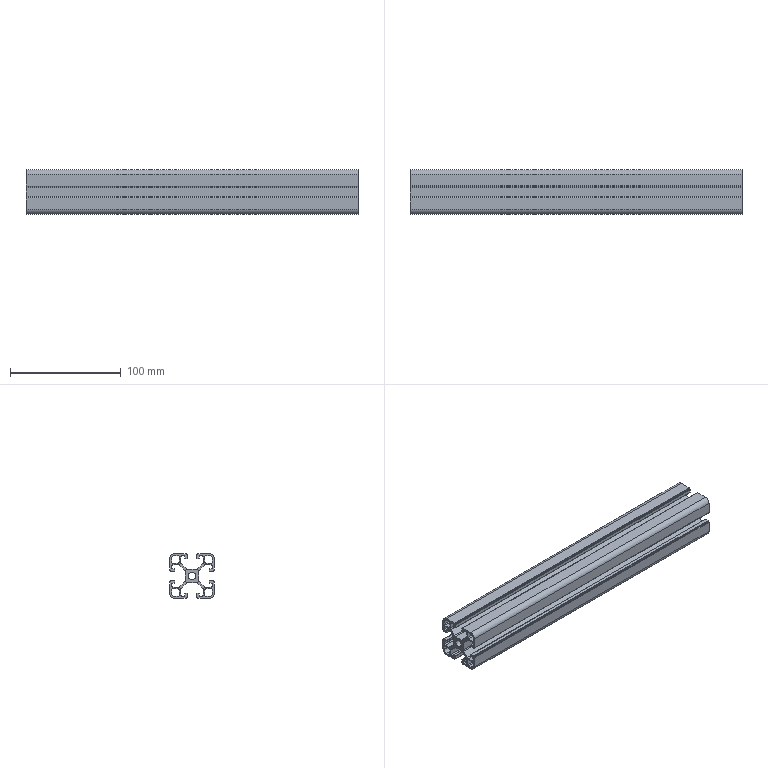Part | STEP file | MK-8-4040C-L-00 profile 4040C standard type 400mm | 1 solid | 188 faces | box 300 x 40 x 40 mm | volume 143475 mm3 | cylinder 94 | plane 94 | commonest cylinder face diameters 0.6 x30 2 x28 4 x16 0.4 x8 6 x4 9 x4